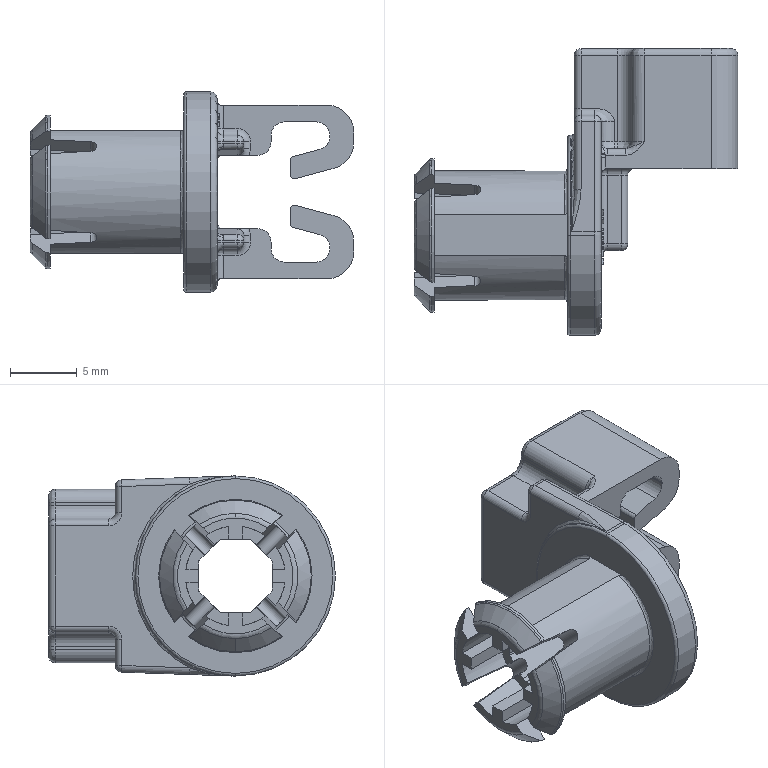Part | STEP file | ZXW735-L-142_1_2_1_1 | 1 solid | 430 faces | box 24.25 x 21.5 x 15 mm | volume 1561 mm3 | plane 186 | cylinder 137 | torus 52 | spline 34 | sphere 16 | cone 5 | commonest cylinder face diameters 1 x90 2 x14 7.5 x8 0.4 x6 0.6 x6 11.5 x5